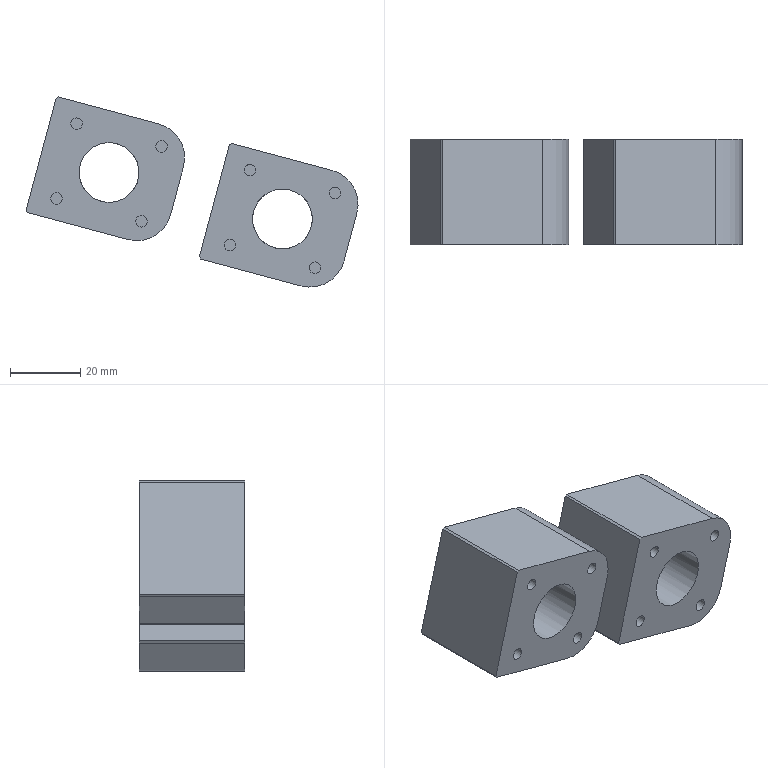Part | NX | 2 solids | 42 faces | box 94.322 x 30 x 54.017 mm | volume 58897 mm3 | plane 26 | cylinder 16 | commonest cylinder face diameters 3.3 x8 20 x4 17 x2 28.04 x2
STEP:
#1=CARTESIAN_POINT('',(618.06,-269.903,-13.791));
#2=VERTEX_POINT('',#1);
#3=CARTESIAN_POINT('',(604.04,-269.903,-13.791));
#4=DIRECTION('',(0.,-1.,0.));
#5=DIRECTION('',(1.,0.,0.000000051));
#6=AXIS2_PLACEMENT_3D('',#3,#4,#5);
#7=CIRCLE('',#6,14.02);
#8=EDGE_CURVE('',#2,#2,#7,.T.);
#9=ORIENTED_EDGE('',*,*,#8,.F.);
#10=EDGE_LOOP('',(#9));
#11=FACE_BOUND('',#10,.T.);
#12=CARTESIAN_POINT('',(612.54,-269.903,-13.791));
#13=VERTEX_POINT('',#12);
#14=CARTESIAN_POINT('',(604.04,-269.903,-13.791));
#15=DIRECTION('',(0.,-1.,0.));
#16=DIRECTION('',(1.,0.,0.));
#17=AXIS2_PLACEMENT_3D('',#14,#15,#16);
#18=CIRCLE('',#17,8.5);
#19=EDGE_CURVE('',#13,#13,#18,.T.);
#20=ORIENTED_EDGE('',*,*,#19,.T.);
#21=EDGE_LOOP('',(#20));
#22=FACE_BOUND('',#21,.T.);
#23=CARTESIAN_POINT('',(604.04,-269.903,-13.791));
#24=DIRECTION('',(0.,-1.,0.));
#25=DIRECTION('',(0.9659,0.,-0.2588));
#26=AXIS2_PLACEMENT_3D('',#23,#24,#25);
#27=PLANE('',#26);
#28=ADVANCED_FACE('',(#11,#22),#27,.F.);
#29=CARTESIAN_POINT('',(590.02,-262.903,-13.791));
#30=VERTEX_POINT('',#29);
#31=CARTESIAN_POINT('',(604.04,-262.903,-13.791));
#32=DIRECTION('',(0.,1.,0.));
#33=DIRECTION('',(-1.,0.,0.));
#34=AXIS2_PLACEMENT_3D('',#31,#32,#33);
#35=CIRCLE('',#34,14.02);
#36=EDGE_CURVE('',#30,#30,#35,.T.);
#37=ORIENTED_EDGE('',*,*,#36,.F.);
#38=EDGE_LOOP('',(#37));
#39=FACE_BOUND('',#38,.T.);
#40=CARTESIAN_POINT('',(589.604,-262.903,7.677));
#41=VERTEX_POINT('',#40);
#42=CARTESIAN_POINT('',(618.099,-262.903,0.04139));
#43=VERTEX_POINT('',#42);
#44=CARTESIAN_POINT('',(154.455,-262.903,124.275));
#45=DIRECTION('',(0.9659,0.,-0.2588));
#46=VECTOR('',#45,1000.);
#47=LINE('',#44,#46);
#48=EDGE_CURVE('',#41,#43,#47,.T.);
#49=ORIENTED_EDGE('',*,*,#48,.T.);
#50=CARTESIAN_POINT('',(625.17,-262.903,-12.206));
#51=VERTEX_POINT('',#50);
#52=CARTESIAN_POINT('',(615.511,-262.903,-9.618));
#53=DIRECTION('',(0.,1.,0.));
#54=DIRECTION('',(-1.,0.,0.));
#55=AXIS2_PLACEMENT_3D('',#52,#53,#54);
#56=CIRCLE('',#55,10.);
#57=EDGE_CURVE('',#43,#51,#56,.T.);
#58=ORIENTED_EDGE('',*,*,#57,.T.);
#59=CARTESIAN_POINT('',(621.547,-262.903,-25.729));
#60=VERTEX_POINT('',#59);
#61=CARTESIAN_POINT('',(622.064,-262.903,-23.797));
#62=DIRECTION('',(-0.2588,0.,-0.9659));
#63=VECTOR('',#62,1000.);
#64=LINE('',#61,#63);
#65=EDGE_CURVE('',#51,#60,#64,.T.);
#66=ORIENTED_EDGE('',*,*,#65,.T.);
#67=CARTESIAN_POINT('',(609.299,-262.903,-32.8));
#68=VERTEX_POINT('',#67);
#69=CARTESIAN_POINT('',(611.887,-262.903,-23.141));
#70=DIRECTION('',(0.,1.,0.));
#71=DIRECTION('',(-1.,0.,0.));
#72=AXIS2_PLACEMENT_3D('',#69,#70,#71);
#73=CIRCLE('',#72,10.);
#74=EDGE_CURVE('',#60,#68,#73,.T.);
#75=ORIENTED_EDGE('',*,*,#74,.T.);
#76=CARTESIAN_POINT('',(580.804,-262.903,-25.165));
#77=VERTEX_POINT('',#76);
#78=CARTESIAN_POINT('',(145.655,-262.903,91.433));
#79=DIRECTION('',(-0.9659,0.,0.2588));
#80=VECTOR('',#79,1000.);
#81=LINE('',#78,#80);
#82=EDGE_CURVE('',#68,#77,#81,.T.);
#83=ORIENTED_EDGE('',*,*,#82,.T.);
#84=CARTESIAN_POINT('',(580.451,-262.903,-24.553));
#85=VERTEX_POINT('',#84);
#86=CARTESIAN_POINT('',(417.286,-262.903,258.057));
#87=DIRECTION('',(-0.5,0.,0.866));
#88=VECTOR('',#87,1000.);
#89=LINE('',#86,#88);
#90=EDGE_CURVE('',#77,#85,#89,.T.);
#91=ORIENTED_EDGE('',*,*,#90,.T.);
#92=CARTESIAN_POINT('',(588.992,-262.903,7.323));
#93=VERTEX_POINT('',#92);
#94=CARTESIAN_POINT('',(583.427,-262.903,-13.444));
#95=DIRECTION('',(-0.2588,0.,-0.9659));
#96=VECTOR('',#95,1000.);
#97=LINE('',#94,#96);
#98=EDGE_CURVE('',#93,#85,#97,.T.);
#99=ORIENTED_EDGE('',*,*,#98,.F.);
#100=CARTESIAN_POINT('',(300.258,-262.903,-159.377));
#101=DIRECTION('',(0.866,0.,0.5));
#102=VECTOR('',#101,1000.);
#103=LINE('',#100,#102);
#104=EDGE_CURVE('',#93,#41,#103,.T.);
#105=ORIENTED_EDGE('',*,*,#104,.T.);
#106=EDGE_LOOP('',(#49,#58,#66,#75,#83,#91,#99,#105));
#107=FACE_BOUND('',#106,.T.);
#108=CARTESIAN_POINT('',(148.761,-262.903,103.024));
#109=DIRECTION('',(0.,1.,0.));
#110=DIRECTION('',(-0.9659,0.,0.2588));
#111=AXIS2_PLACEMENT_3D('',#108,#109,#110);
#112=PLANE('',#111);
#113=ADVANCED_FACE('',(#39,#107),#112,.T.);
#114=CARTESIAN_POINT('',(594.386,-292.903,-1.525));
#115=VERTEX_POINT('',#114);
#116=CARTESIAN_POINT('',(594.813,-292.903,0.06927));
#117=DIRECTION('',(0.,1.,0.));
#118=DIRECTION('',(-0.2588,0.,-0.9659));
#119=AXIS2_PLACEMENT_3D('',#116,#117,#118);
#120=CIRCLE('',#119,1.65);
#121=EDGE_CURVE('',#115,#115,#120,.T.);
#122=ORIENTED_EDGE('',*,*,#121,.T.);
#123=EDGE_LOOP('',(#122));
#124=FACE_BOUND('',#123,.T.);
#125=CARTESIAN_POINT('',(588.692,-292.903,-22.775));
#126=VERTEX_POINT('',#125);
#127=CARTESIAN_POINT('',(589.119,-292.903,-21.181));
#128=DIRECTION('',(0.,1.,0.));
#129=DIRECTION('',(-0.2588,0.,-0.9659));
#130=AXIS2_PLACEMENT_3D('',#127,#128,#129);
#131=CIRCLE('',#130,1.65);
#132=EDGE_CURVE('',#126,#126,#131,.T.);
#133=ORIENTED_EDGE('',*,*,#132,.T.);
#134=EDGE_LOOP('',(#133));
#135=FACE_BOUND('',#134,.T.);
#136=CARTESIAN_POINT('',(618.534,-292.903,-7.995));
#137=VERTEX_POINT('',#136);
#138=CARTESIAN_POINT('',(618.961,-292.903,-6.401));
#139=DIRECTION('',(0.,1.,0.));
#140=DIRECTION('',(-0.2588,0.,-0.9659));
#141=AXIS2_PLACEMENT_3D('',#138,#139,#140);
#142=CIRCLE('',#141,1.65);
#143=EDGE_CURVE('',#137,#137,#142,.T.);
#144=ORIENTED_EDGE('',*,*,#143,.T.);
#145=EDGE_LOOP('',(#144));
#146=FACE_BOUND('',#145,.T.);
#147=CARTESIAN_POINT('',(612.84,-292.903,-29.245));
#148=VERTEX_POINT('',#147);
#149=CARTESIAN_POINT('',(613.267,-292.903,-27.652));
#150=DIRECTION('',(0.,1.,0.));
#151=DIRECTION('',(-0.2588,0.,-0.9659));
#152=AXIS2_PLACEMENT_3D('',#149,#150,#151);
#153=CIRCLE('',#152,1.65);
#154=EDGE_CURVE('',#148,#148,#153,.T.);
#155=ORIENTED_EDGE('',*,*,#154,.T.);
#156=EDGE_LOOP('',(#155));
#157=FACE_BOUND('',#156,.T.);
#158=CARTESIAN_POINT('',(618.099,-292.903,0.04139));
#159=VERTEX_POINT('',#158);
#160=CARTESIAN_POINT('',(625.17,-292.903,-12.206));
#161=VERTEX_POINT('',#160);
#162=CARTESIAN_POINT('',(615.511,-292.903,-9.618));
#163=DIRECTION('',(0.,1.,0.));
#164=DIRECTION('',(0.,0.,1.));
#165=AXIS2_PLACEMENT_3D('',#162,#163,#164);
#166=CIRCLE('',#165,10.);
#167=EDGE_CURVE('',#159,#161,#166,.T.);
#168=ORIENTED_EDGE('',*,*,#167,.F.);
#169=CARTESIAN_POINT('',(589.604,-292.903,7.677));
#170=VERTEX_POINT('',#169);
#171=CARTESIAN_POINT('',(572.218,-292.903,12.335));
#172=DIRECTION('',(0.9659,0.,-0.2588));
#173=VECTOR('',#172,1000.);
#174=LINE('',#171,#173);
#175=EDGE_CURVE('',#170,#159,#174,.T.);
#176=ORIENTED_EDGE('',*,*,#175,.F.);
#177=CARTESIAN_POINT('',(588.992,-292.903,7.323));
#178=VERTEX_POINT('',#177);
#179=CARTESIAN_POINT('',(568.171,-292.903,-4.698));
#180=DIRECTION('',(0.866,0.,0.5));
#181=VECTOR('',#180,1000.);
#182=LINE('',#179,#181);
#183=EDGE_CURVE('',#178,#170,#182,.T.);
#184=ORIENTED_EDGE('',*,*,#183,.F.);
#185=CARTESIAN_POINT('',(580.451,-292.903,-24.553));
#186=VERTEX_POINT('',#185);
#187=CARTESIAN_POINT('',(584.721,-292.903,-8.615));
#188=DIRECTION('',(-0.2588,0.,-0.9659));
#189=VECTOR('',#188,1000.);
#190=LINE('',#187,#189);
#191=EDGE_CURVE('',#178,#186,#190,.T.);
#192=ORIENTED_EDGE('',*,*,#191,.T.);
#193=CARTESIAN_POINT('',(580.804,-292.903,-25.165));
#194=VERTEX_POINT('',#193);
#195=CARTESIAN_POINT('',(568.43,-292.903,-3.732));
#196=DIRECTION('',(-0.5,0.,0.866));
#197=VECTOR('',#196,1000.);
#198=LINE('',#195,#197);
#199=EDGE_CURVE('',#194,#186,#198,.T.);
#200=ORIENTED_EDGE('',*,*,#199,.F.);
#201=CARTESIAN_POINT('',(609.299,-292.903,-32.8));
#202=VERTEX_POINT('',#201);
#203=CARTESIAN_POINT('',(563.418,-292.903,-20.506));
#204=DIRECTION('',(-0.9659,0.,0.2588));
#205=VECTOR('',#204,1000.);
#206=LINE('',#203,#205);
#207=EDGE_CURVE('',#202,#194,#206,.T.);
#208=ORIENTED_EDGE('',*,*,#207,.F.);
#209=CARTESIAN_POINT('',(621.547,-292.903,-25.729));
#210=VERTEX_POINT('',#209);
#211=CARTESIAN_POINT('',(611.887,-292.903,-23.141));
#212=DIRECTION('',(0.,1.,0.));
#213=DIRECTION('',(0.,0.,1.));
#214=AXIS2_PLACEMENT_3D('',#211,#212,#213);
#215=CIRCLE('',#214,10.);
#216=EDGE_CURVE('',#210,#202,#215,.T.);
#217=ORIENTED_EDGE('',*,*,#216,.F.);
#218=CARTESIAN_POINT('',(623.358,-292.903,-18.968));
#219=DIRECTION('',(-0.2588,0.,-0.9659));
#220=VECTOR('',#219,1000.);
#221=LINE('',#218,#220);
#222=EDGE_CURVE('',#161,#210,#221,.T.);
#223=ORIENTED_EDGE('',*,*,#222,.F.);
#224=EDGE_LOOP('',(#168,#176,#184,#192,#200,#208,#217,#223));
#225=FACE_BOUND('',#224,.T.);
#226=CARTESIAN_POINT('',(604.04,-292.903,-5.291));
#227=VERTEX_POINT('',#226);
#228=CARTESIAN_POINT('',(604.04,-292.903,-13.791));
#229=DIRECTION('',(0.,1.,0.));
#230=DIRECTION('',(0.,0.,1.));
#231=AXIS2_PLACEMENT_3D('',#228,#229,#230);
#232=CIRCLE('',#231,8.5);
#233=EDGE_CURVE('',#227,#227,#232,.T.);
#234=ORIENTED_EDGE('',*,*,#233,.T.);
#235=EDGE_LOOP('',(#234));
#236=FACE_BOUND('',#235,.T.);
#237=CARTESIAN_POINT('',(567.818,-292.903,-4.085));
#238=DIRECTION('',(0.,1.,0.));
#239=DIRECTION('',(-0.2588,0.,-0.9659));
#240=AXIS2_PLACEMENT_3D('',#237,#238,#239);
#241=PLANE('',#240);
#242=ADVANCED_FACE('',(#124,#135,#146,#157,#225,#236),#241,.F.);
#243=ORIENTED_EDGE('',*,*,#57,.F.);
#244=CARTESIAN_POINT('',(618.099,-277.903,0.04139));
#245=DIRECTION('',(0.,-1.,0.));
#246=VECTOR('',#245,1000.);
#247=LINE('',#244,#246);
#248=EDGE_CURVE('',#43,#159,#247,.T.);
#249=ORIENTED_EDGE('',*,*,#248,.T.);
#250=ORIENTED_EDGE('',*,*,#167,.T.);
#251=CARTESIAN_POINT('',(625.17,-279.903,-12.206));
#252=DIRECTION('',(0.,1.,0.));
#253=VECTOR('',#252,1000.);
#254=LINE('',#251,#253);
#255=EDGE_CURVE('',#161,#51,#254,.T.);
#256=ORIENTED_EDGE('',*,*,#255,.T.);
#257=EDGE_LOOP('',(#243,#249,#250,#256));
#258=FACE_BOUND('',#257,.T.);
#259=CARTESIAN_POINT('',(615.511,-279.903,-9.618));
#260=DIRECTION('',(0.,1.,0.));
#261=DIRECTION('',(0.9659,0.,-0.2588));
#262=AXIS2_PLACEMENT_3D('',#259,#260,#261);
#263=CYLINDRICAL_SURFACE('',#262,10.);
#264=ADVANCED_FACE('',(#258),#263,.T.);
#265=ORIENTED_EDGE('',*,*,#65,.F.);
#266=ORIENTED_EDGE('',*,*,#255,.F.);
#267=ORIENTED_EDGE('',*,*,#222,.T.);
#268=CARTESIAN_POINT('',(621.547,-279.903,-25.729));
#269=DIRECTION('',(0.,-1.,0.));
#270=VECTOR('',#269,1000.);
#271=LINE('',#268,#270);
#272=EDGE_CURVE('',#60,#210,#271,.T.);
#273=ORIENTED_EDGE('',*,*,#272,.F.);
#274=EDGE_LOOP('',(#265,#266,#267,#273));
#275=FACE_BOUND('',#274,.T.);
#276=CARTESIAN_POINT('',(622.064,-279.903,-23.797));
#277=DIRECTION('',(0.9659,0.,-0.2588));
#278=DIRECTION('',(0.,1.,0.));
#279=AXIS2_PLACEMENT_3D('',#276,#277,#278);
#280=PLANE('',#279);
#281=ADVANCED_FACE('',(#275),#280,.T.);
#282=ORIENTED_EDGE('',*,*,#74,.F.);
#283=ORIENTED_EDGE('',*,*,#272,.T.);
#284=ORIENTED_EDGE('',*,*,#216,.T.);
#285=CARTESIAN_POINT('',(609.299,-277.903,-32.8));
#286=DIRECTION('',(0.,1.,0.));
#287=VECTOR('',#286,1000.);
#288=LINE('',#285,#287);
#289=EDGE_CURVE('',#202,#68,#288,.T.);
#290=ORIENTED_EDGE('',*,*,#289,.T.);
#291=EDGE_LOOP('',(#282,#283,#284,#290));
#292=FACE_BOUND('',#291,.T.);
#293=CARTESIAN_POINT('',(611.887,-279.903,-23.141));
#294=DIRECTION('',(0.,-1.,0.));
#295=DIRECTION('',(-0.9659,0.,0.2588));
#296=AXIS2_PLACEMENT_3D('',#293,#294,#295);
#297=CYLINDRICAL_SURFACE('',#296,10.);
#298=ADVANCED_FACE('',(#292),#297,.T.);
#299=ORIENTED_EDGE('',*,*,#82,.F.);
#300=ORIENTED_EDGE('',*,*,#289,.F.);
#301=ORIENTED_EDGE('',*,*,#207,.T.);
#302=CARTESIAN_POINT('',(580.804,-262.903,-25.165));
#303=DIRECTION('',(0.,1.,0.));
#304=VECTOR('',#303,1000.);
#305=LINE('',#302,#304);
#306=EDGE_CURVE('',#194,#77,#305,.T.);
#307=ORIENTED_EDGE('',*,*,#306,.T.);
#308=EDGE_LOOP('',(#299,#300,#301,#307));
#309=FACE_BOUND('',#308,.T.);
#310=CARTESIAN_POINT('',(383.273,-277.903,27.764));
#311=DIRECTION('',(-0.2588,0.,-0.9659));
#312=DIRECTION('',(0.,-1.,0.));
#313=AXIS2_PLACEMENT_3D('',#310,#311,#312);
#314=PLANE('',#313);
#315=ADVANCED_FACE('',(#309),#314,.T.);
#316=ORIENTED_EDGE('',*,*,#90,.F.);
#317=ORIENTED_EDGE('',*,*,#306,.F.);
#318=ORIENTED_EDGE('',*,*,#199,.T.);
#319=CARTESIAN_POINT('',(580.451,-292.903,-24.553));
#320=DIRECTION('',(0.,-1.,0.));
#321=VECTOR('',#320,1000.);
#322=LINE('',#319,#321);
#323=EDGE_CURVE('',#85,#186,#322,.T.);
#324=ORIENTED_EDGE('',*,*,#323,.F.);
#325=EDGE_LOOP('',(#316,#317,#318,#324));
#326=FACE_BOUND('',#325,.T.);
#327=CARTESIAN_POINT('',(580.451,-269.903,-24.553));
#328=DIRECTION('',(-0.866,0.,-0.5));
#329=DIRECTION('',(0.,1.,0.));
#330=AXIS2_PLACEMENT_3D('',#327,#328,#329);
#331=PLANE('',#330);
#332=ADVANCED_FACE('',(#326),#331,.T.);
#333=CARTESIAN_POINT('',(588.992,-262.903,7.323));
#334=DIRECTION('',(0.,1.,0.));
#335=VECTOR('',#334,1000.);
#336=LINE('',#333,#335);
#337=EDGE_CURVE('',#178,#93,#336,.T.);
#338=ORIENTED_EDGE('',*,*,#337,.T.);
#339=ORIENTED_EDGE('',*,*,#98,.T.);
#340=ORIENTED_EDGE('',*,*,#323,.T.);
#341=ORIENTED_EDGE('',*,*,#191,.F.);
#342=EDGE_LOOP('',(#338,#339,#340,#341));
#343=FACE_BOUND('',#342,.T.);
#344=CARTESIAN_POINT('',(584.721,-269.903,-8.615));
#345=DIRECTION('',(0.9659,0.,-0.2588));
#346=DIRECTION('',(0.2588,0.,0.9659));
#347=AXIS2_PLACEMENT_3D('',#344,#345,#346);
#348=PLANE('',#347);
#349=ADVANCED_FACE('',(#343),#348,.F.);
#350=ORIENTED_EDGE('',*,*,#104,.F.);
#351=ORIENTED_EDGE('',*,*,#337,.F.);
#352=ORIENTED_EDGE('',*,*,#183,.T.);
#353=CARTESIAN_POINT('',(589.604,-292.903,7.677));
#354=DIRECTION('',(0.,-1.,0.));
#355=VECTOR('',#354,1000.);
#356=LINE('',#353,#355);
#357=EDGE_CURVE('',#41,#170,#356,.T.);
#358=ORIENTED_EDGE('',*,*,#357,.F.);
#359=EDGE_LOOP('',(#350,#351,#352,#358));
#360=FACE_BOUND('',#359,.T.);
#361=CARTESIAN_POINT('',(589.604,-277.903,7.677));
#362=DIRECTION('',(-0.5,0.,0.866));
#363=DIRECTION('',(0.,1.,0.));
#364=AXIS2_PLACEMENT_3D('',#361,#362,#363);
#365=PLANE('',#364);
#366=ADVANCED_FACE('',(#360),#365,.T.);
#367=ORIENTED_EDGE('',*,*,#48,.F.);
#368=ORIENTED_EDGE('',*,*,#357,.T.);
#369=ORIENTED_EDGE('',*,*,#175,.T.);
#370=ORIENTED_EDGE('',*,*,#248,.F.);
#371=EDGE_LOOP('',(#367,#368,#369,#370));
#372=FACE_BOUND('',#371,.T.);
#373=CARTESIAN_POINT('',(392.072,-277.903,60.605));
#374=DIRECTION('',(0.2588,0.,0.9659));
#375=DIRECTION('',(0.,1.,0.));
#376=AXIS2_PLACEMENT_3D('',#373,#374,#375);
#377=PLANE('',#376);
#378=ADVANCED_FACE('',(#372),#377,.T.);
#379=ORIENTED_EDGE('',*,*,#121,.F.);
#380=EDGE_LOOP('',(#379));
#381=FACE_BOUND('',#380,.T.);
#382=CARTESIAN_POINT('',(594.813,-277.903,1.719));
#383=VERTEX_POINT('',#382);
#384=CARTESIAN_POINT('',(594.813,-277.903,0.06927));
#385=DIRECTION('',(0.,-1.,0.));
#386=DIRECTION('',(0.,0.,1.));
#387=AXIS2_PLACEMENT_3D('',#384,#385,#386);
#388=CIRCLE('',#387,1.65);
#389=EDGE_CURVE('',#383,#383,#388,.T.);
#390=ORIENTED_EDGE('',*,*,#389,.F.);
#391=EDGE_LOOP('',(#390));
#392=FACE_BOUND('',#391,.T.);
#393=CARTESIAN_POINT('',(594.813,-292.903,0.06927));
#394=DIRECTION('',(0.,1.,0.));
#395=DIRECTION('',(-0.2588,0.,-0.9659));
#396=AXIS2_PLACEMENT_3D('',#393,#394,#395);
#397=CYLINDRICAL_SURFACE('',#396,1.65);
#398=ADVANCED_FACE('',(#381,#392),#397,.F.);
#399=ORIENTED_EDGE('',*,*,#389,.T.);
#400=EDGE_LOOP('',(#399));
#401=FACE_BOUND('',#400,.T.);
#402=CARTESIAN_POINT('',(589.119,-277.903,-21.181));
#403=DIRECTION('',(0.,1.,0.));
#404=DIRECTION('',(-0.2588,0.,-0.9659));
#405=AXIS2_PLACEMENT_3D('',#402,#403,#404);
#406=PLANE('',#405);
#407=ADVANCED_FACE('',(#401),#406,.F.);
#408=ORIENTED_EDGE('',*,*,#132,.F.);
#409=EDGE_LOOP('',(#408));
#410=FACE_BOUND('',#409,.T.);
#411=CARTESIAN_POINT('',(588.692,-277.903,-22.775));
#412=VERTEX_POINT('',#411);
#413=CARTESIAN_POINT('',(589.119,-277.903,-21.181));
#414=DIRECTION('',(0.,-1.,0.));
#415=DIRECTION('',(-0.2588,0.,-0.9659));
#416=AXIS2_PLACEMENT_3D('',#413,#414,#415);
#417=CIRCLE('',#416,1.65);
#418=EDGE_CURVE('',#412,#412,#417,.T.);
#419=ORIENTED_EDGE('',*,*,#418,.F.);
#420=EDGE_LOOP('',(#419));
#421=FACE_BOUND('',#420,.T.);
#422=CARTESIAN_POINT('',(589.119,-292.903,-21.181));
#423=DIRECTION('',(0.,1.,0.));
#424=DIRECTION('',(-0.2588,0.,-0.9659));
#425=AXIS2_PLACEMENT_3D('',#422,#423,#424);
#426=CYLINDRICAL_SURFACE('',#425,1.65);
#427=ADVANCED_FACE('',(#410,#421),#426,.F.);
#428=ORIENTED_EDGE('',*,*,#418,.T.);
#429=EDGE_LOOP('',(#428));
#430=FACE_BOUND('',#429,.T.);
#431=CARTESIAN_POINT('',(589.119,-277.903,-21.181));
#432=DIRECTION('',(0.,1.,0.));
#433=DIRECTION('',(-0.2588,0.,-0.9659));
#434=AXIS2_PLACEMENT_3D('',#431,#432,#433);
#435=PLANE('',#434);
#436=ADVANCED_FACE('',(#430),#435,.F.);
#437=ORIENTED_EDGE('',*,*,#143,.F.);
#438=EDGE_LOOP('',(#437));
#439=FACE_BOUND('',#438,.T.);
#440=CARTESIAN_POINT('',(618.961,-277.903,-4.751));
#441=VERTEX_POINT('',#440);
#442=CARTESIAN_POINT('',(618.961,-277.903,-6.401));
#443=DIRECTION('',(0.,-1.,0.));
#444=DIRECTION('',(0.,0.,1.));
#445=AXIS2_PLACEMENT_3D('',#442,#443,#444);
#446=CIRCLE('',#445,1.65);
#447=EDGE_CURVE('',#441,#441,#446,.T.);
#448=ORIENTED_EDGE('',*,*,#447,.F.);
#449=EDGE_LOOP('',(#448));
#450=FACE_BOUND('',#449,.T.);
#451=CARTESIAN_POINT('',(618.961,-292.903,-6.401));
#452=DIRECTION('',(0.,1.,0.));
#453=DIRECTION('',(-0.2588,0.,-0.9659));
#454=AXIS2_PLACEMENT_3D('',#451,#452,#453);
#455=CYLINDRICAL_SURFACE('',#454,1.65);
#456=ADVANCED_FACE('',(#439,#450),#455,.F.);
#457=ORIENTED_EDGE('',*,*,#447,.T.);
#458=EDGE_LOOP('',(#457));
#459=FACE_BOUND('',#458,.T.);
#460=CARTESIAN_POINT('',(589.119,-277.903,-21.181));
#461=DIRECTION('',(0.,1.,0.));
#462=DIRECTION('',(-0.2588,0.,-0.9659));
#463=AXIS2_PLACEMENT_3D('',#460,#461,#462);
#464=PLANE('',#463);
#465=ADVANCED_FACE('',(#459),#464,.F.);
#466=ORIENTED_EDGE('',*,*,#154,.F.);
#467=EDGE_LOOP('',(#466));
#468=FACE_BOUND('',#467,.T.);
#469=CARTESIAN_POINT('',(613.267,-277.903,-26.002));
#470=VERTEX_POINT('',#469);
#471=CARTESIAN_POINT('',(613.267,-277.903,-27.652));
#472=DIRECTION('',(0.,-1.,0.));
#473=DIRECTION('',(0.,0.,1.));
#474=AXIS2_PLACEMENT_3D('',#471,#472,#473);
#475=CIRCLE('',#474,1.65);
#476=EDGE_CURVE('',#470,#470,#475,.T.);
#477=ORIENTED_EDGE('',*,*,#476,.F.);
#478=EDGE_LOOP('',(#477));
#479=FACE_BOUND('',#478,.T.);
#480=CARTESIAN_POINT('',(613.267,-292.903,-27.652));
#481=DIRECTION('',(0.,1.,0.));
#482=DIRECTION('',(-0.2588,0.,-0.9659));
#483=AXIS2_PLACEMENT_3D('',#480,#481,#482);
#484=CYLINDRICAL_SURFACE('',#483,1.65);
#485=ADVANCED_FACE('',(#468,#479),#484,.F.);
#486=ORIENTED_EDGE('',*,*,#476,.T.);
#487=EDGE_LOOP('',(#486));
#488=FACE_BOUND('',#487,.T.);
#489=CARTESIAN_POINT('',(589.119,-277.903,-21.181));
#490=DIRECTION('',(0.,1.,0.));
#491=DIRECTION('',(-0.2588,0.,-0.9659));
#492=AXIS2_PLACEMENT_3D('',#489,#490,#491);
#493=PLANE('',#492);
#494=ADVANCED_FACE('',(#488),#493,.F.);
#495=ORIENTED_EDGE('',*,*,#233,.F.);
#496=EDGE_LOOP('',(#495));
#497=FACE_BOUND('',#496,.T.);
#498=ORIENTED_EDGE('',*,*,#19,.F.);
#499=EDGE_LOOP('',(#498));
#500=FACE_BOUND('',#499,.T.);
#501=CARTESIAN_POINT('',(604.04,-284.903,-13.791));
#502=DIRECTION('',(0.,-1.,0.));
#503=DIRECTION('',(0.2588,0.,0.9659));
#504=AXIS2_PLACEMENT_3D('',#501,#502,#503);
#505=CYLINDRICAL_SURFACE('',#504,8.5);
#506=ADVANCED_FACE('',(#497,#500),#505,.F.);
#507=ORIENTED_EDGE('',*,*,#8,.T.);
#508=EDGE_LOOP('',(#507));
#509=FACE_BOUND('',#508,.T.);
#510=ORIENTED_EDGE('',*,*,#36,.T.);
#511=EDGE_LOOP('',(#510));
#512=FACE_BOUND('',#511,.T.);
#513=CARTESIAN_POINT('',(604.04,-269.903,-13.791));
#514=DIRECTION('',(0.,1.,0.));
#515=DIRECTION('',(-0.2588,0.,-0.9659));
#516=AXIS2_PLACEMENT_3D('',#513,#514,#515);
#517=CYLINDRICAL_SURFACE('',#516,14.02);
#518=ADVANCED_FACE('',(#509,#512),#517,.F.);
#519=CLOSED_SHELL('',(#28,#113,#242,#264,#281,#298,#315,#332,#349,#366,#378,#398,#407,#427,#436,#456,#465,#485,#494,#506,#518));
#520=MANIFOLD_SOLID_BREP('',#519);
#521=CARTESIAN_POINT('',(568.798,-269.903,-0.5914));
#522=VERTEX_POINT('',#521);
#523=CARTESIAN_POINT('',(554.778,-269.903,-0.5914));
#524=DIRECTION('',(0.,-1.,0.));
#525=DIRECTION('',(1.,0.,0.000000051));
#526=AXIS2_PLACEMENT_3D('',#523,#524,#525);
#527=CIRCLE('',#526,14.02);
#528=EDGE_CURVE('',#522,#522,#527,.T.);
#529=ORIENTED_EDGE('',*,*,#528,.F.);
#530=EDGE_LOOP('',(#529));
#531=FACE_BOUND('',#530,.T.);
#532=CARTESIAN_POINT('',(563.278,-269.903,-0.5914));
#533=VERTEX_POINT('',#532);
#534=CARTESIAN_POINT('',(554.778,-269.903,-0.5914));
#535=DIRECTION('',(0.,-1.,0.));
#536=DIRECTION('',(1.,0.,0.));
#537=AXIS2_PLACEMENT_3D('',#534,#535,#536);
#538=CIRCLE('',#537,8.5);
#539=EDGE_CURVE('',#533,#533,#538,.T.);
#540=ORIENTED_EDGE('',*,*,#539,.T.);
#541=EDGE_LOOP('',(#540));
#542=FACE_BOUND('',#541,.T.);
#543=CARTESIAN_POINT('',(554.778,-269.903,-0.5914));
#544=DIRECTION('',(0.,-1.,0.));
#545=DIRECTION('',(0.9659,0.,-0.2588));
#546=AXIS2_PLACEMENT_3D('',#543,#544,#545);
#547=PLANE('',#546);
#548=ADVANCED_FACE('',(#531,#542),#547,.F.);
#549=CARTESIAN_POINT('',(540.758,-262.903,-0.5914));
#550=VERTEX_POINT('',#549);
#551=CARTESIAN_POINT('',(554.778,-262.903,-0.5914));
#552=DIRECTION('',(0.,1.,0.));
#553=DIRECTION('',(-1.,0.,0.));
#554=AXIS2_PLACEMENT_3D('',#551,#552,#553);
#555=CIRCLE('',#554,14.02);
#556=EDGE_CURVE('',#550,#550,#555,.T.);
#557=ORIENTED_EDGE('',*,*,#556,.F.);
#558=EDGE_LOOP('',(#557));
#559=FACE_BOUND('',#558,.T.);
#560=CARTESIAN_POINT('',(540.342,-262.903,20.876));
#561=VERTEX_POINT('',#560);
#562=CARTESIAN_POINT('',(568.837,-262.903,13.241));
#563=VERTEX_POINT('',#562);
#564=CARTESIAN_POINT('',(105.193,-262.903,137.474));
#565=DIRECTION('',(0.9659,0.,-0.2588));
#566=VECTOR('',#565,1000.);
#567=LINE('',#564,#566);
#568=EDGE_CURVE('',#561,#563,#567,.T.);
#569=ORIENTED_EDGE('',*,*,#568,.T.);
#570=CARTESIAN_POINT('',(575.908,-262.903,0.9937));
#571=VERTEX_POINT('',#570);
#572=CARTESIAN_POINT('',(566.249,-262.903,3.582));
#573=DIRECTION('',(0.,1.,0.));
#574=DIRECTION('',(-1.,0.,0.));
#575=AXIS2_PLACEMENT_3D('',#572,#573,#574);
#576=CIRCLE('',#575,10.);
#577=EDGE_CURVE('',#563,#571,#576,.T.);
#578=ORIENTED_EDGE('',*,*,#577,.T.);
#579=CARTESIAN_POINT('',(572.285,-262.903,-12.529));
#580=VERTEX_POINT('',#579);
#581=CARTESIAN_POINT('',(572.802,-262.903,-10.597));
#582=DIRECTION('',(-0.2588,0.,-0.9659));
#583=VECTOR('',#582,1000.);
#584=LINE('',#581,#583);
#585=EDGE_CURVE('',#571,#580,#584,.T.);
#586=ORIENTED_EDGE('',*,*,#585,.T.);
#587=CARTESIAN_POINT('',(560.037,-262.903,-19.6));
#588=VERTEX_POINT('',#587);
#589=CARTESIAN_POINT('',(562.625,-262.903,-9.941));
#590=DIRECTION('',(0.,1.,0.));
#591=DIRECTION('',(-1.,0.,0.));
#592=AXIS2_PLACEMENT_3D('',#589,#590,#591);
#593=CIRCLE('',#592,10.);
#594=EDGE_CURVE('',#580,#588,#593,.T.);
#595=ORIENTED_EDGE('',*,*,#594,.T.);
#596=CARTESIAN_POINT('',(531.542,-262.903,-11.965));
#597=VERTEX_POINT('',#596);
#598=CARTESIAN_POINT('',(96.393,-262.903,104.633));
#599=DIRECTION('',(-0.9659,0.,0.2588));
#600=VECTOR('',#599,1000.);
#601=LINE('',#598,#600);
#602=EDGE_CURVE('',#588,#597,#601,.T.);
#603=ORIENTED_EDGE('',*,*,#602,.T.);
#604=CARTESIAN_POINT('',(531.189,-262.903,-11.353));
#605=VERTEX_POINT('',#604);
#606=CARTESIAN_POINT('',(368.024,-262.903,271.257));
#607=DIRECTION('',(-0.5,0.,0.866));
#608=VECTOR('',#607,1000.);
#609=LINE('',#606,#608);
#610=EDGE_CURVE('',#597,#605,#609,.T.);
#611=ORIENTED_EDGE('',*,*,#610,.T.);
#612=CARTESIAN_POINT('',(539.73,-262.903,20.523));
#613=VERTEX_POINT('',#612);
#614=CARTESIAN_POINT('',(534.165,-262.903,-0.2446));
#615=DIRECTION('',(-0.2588,0.,-0.9659));
#616=VECTOR('',#615,1000.);
#617=LINE('',#614,#616);
#618=EDGE_CURVE('',#613,#605,#617,.T.);
#619=ORIENTED_EDGE('',*,*,#618,.F.);
#620=CARTESIAN_POINT('',(250.996,-262.903,-146.178));
#621=DIRECTION('',(0.866,0.,0.5));
#622=VECTOR('',#621,1000.);
#623=LINE('',#620,#622);
#624=EDGE_CURVE('',#613,#561,#623,.T.);
#625=ORIENTED_EDGE('',*,*,#624,.T.);
#626=EDGE_LOOP('',(#569,#578,#586,#595,#603,#611,#619,#625));
#627=FACE_BOUND('',#626,.T.);
#628=CARTESIAN_POINT('',(99.499,-262.903,116.224));
#629=DIRECTION('',(0.,1.,0.));
#630=DIRECTION('',(-0.9659,0.,0.2588));
#631=AXIS2_PLACEMENT_3D('',#628,#629,#630);
#632=PLANE('',#631);
#633=ADVANCED_FACE('',(#559,#627),#632,.T.);
#634=CARTESIAN_POINT('',(545.124,-292.903,11.675));
#635=VERTEX_POINT('',#634);
#636=CARTESIAN_POINT('',(545.551,-292.903,13.269));
#637=DIRECTION('',(0.,1.,0.));
#638=DIRECTION('',(-0.2588,0.,-0.9659));
#639=AXIS2_PLACEMENT_3D('',#636,#637,#638);
#640=CIRCLE('',#639,1.65);
#641=EDGE_CURVE('',#635,#635,#640,.T.);
#642=ORIENTED_EDGE('',*,*,#641,.T.);
#643=EDGE_LOOP('',(#642));
#644=FACE_BOUND('',#643,.T.);
#645=CARTESIAN_POINT('',(539.43,-292.903,-9.575));
#646=VERTEX_POINT('',#645);
#647=CARTESIAN_POINT('',(539.857,-292.903,-7.981));
#648=DIRECTION('',(0.,1.,0.));
#649=DIRECTION('',(-0.2588,0.,-0.9659));
#650=AXIS2_PLACEMENT_3D('',#647,#648,#649);
#651=CIRCLE('',#650,1.65);
#652=EDGE_CURVE('',#646,#646,#651,.T.);
#653=ORIENTED_EDGE('',*,*,#652,.T.);
#654=EDGE_LOOP('',(#653));
#655=FACE_BOUND('',#654,.T.);
#656=CARTESIAN_POINT('',(569.272,-292.903,5.205));
#657=VERTEX_POINT('',#656);
#658=CARTESIAN_POINT('',(569.699,-292.903,6.799));
#659=DIRECTION('',(0.,1.,0.));
#660=DIRECTION('',(-0.2588,0.,-0.9659));
#661=AXIS2_PLACEMENT_3D('',#658,#659,#660);
#662=CIRCLE('',#661,1.65);
#663=EDGE_CURVE('',#657,#657,#662,.T.);
#664=ORIENTED_EDGE('',*,*,#663,.T.);
#665=EDGE_LOOP('',(#664));
#666=FACE_BOUND('',#665,.T.);
#667=CARTESIAN_POINT('',(563.578,-292.903,-16.046));
#668=VERTEX_POINT('',#667);
#669=CARTESIAN_POINT('',(564.005,-292.903,-14.452));
#670=DIRECTION('',(0.,1.,0.));
#671=DIRECTION('',(-0.2588,0.,-0.9659));
#672=AXIS2_PLACEMENT_3D('',#669,#670,#671);
#673=CIRCLE('',#672,1.65);
#674=EDGE_CURVE('',#668,#668,#673,.T.);
#675=ORIENTED_EDGE('',*,*,#674,.T.);
#676=EDGE_LOOP('',(#675));
#677=FACE_BOUND('',#676,.T.);
#678=CARTESIAN_POINT('',(568.837,-292.903,13.241));
#679=VERTEX_POINT('',#678);
#680=CARTESIAN_POINT('',(575.908,-292.903,0.9937));
#681=VERTEX_POINT('',#680);
#682=CARTESIAN_POINT('',(566.249,-292.903,3.582));
#683=DIRECTION('',(0.,1.,0.));
#684=DIRECTION('',(0.,0.,1.));
#685=AXIS2_PLACEMENT_3D('',#682,#683,#684);
#686=CIRCLE('',#685,10.);
#687=EDGE_CURVE('',#679,#681,#686,.T.);
#688=ORIENTED_EDGE('',*,*,#687,.F.);
#689=CARTESIAN_POINT('',(540.342,-292.903,20.876));
#690=VERTEX_POINT('',#689);
#691=CARTESIAN_POINT('',(522.955,-292.903,25.535));
#692=DIRECTION('',(0.9659,0.,-0.2588));
#693=VECTOR('',#692,1000.);
#694=LINE('',#691,#693);
#695=EDGE_CURVE('',#690,#679,#694,.T.);
#696=ORIENTED_EDGE('',*,*,#695,.F.);
#697=CARTESIAN_POINT('',(539.73,-292.903,20.523));
#698=VERTEX_POINT('',#697);
#699=CARTESIAN_POINT('',(518.909,-292.903,8.502));
#700=DIRECTION('',(0.866,0.,0.5));
#701=VECTOR('',#700,1000.);
#702=LINE('',#699,#701);
#703=EDGE_CURVE('',#698,#690,#702,.T.);
#704=ORIENTED_EDGE('',*,*,#703,.F.);
#705=CARTESIAN_POINT('',(531.189,-292.903,-11.353));
#706=VERTEX_POINT('',#705);
#707=CARTESIAN_POINT('',(535.459,-292.903,4.585));
#708=DIRECTION('',(-0.2588,0.,-0.9659));
#709=VECTOR('',#708,1000.);
#710=LINE('',#707,#709);
#711=EDGE_CURVE('',#698,#706,#710,.T.);
#712=ORIENTED_EDGE('',*,*,#711,.T.);
#713=CARTESIAN_POINT('',(531.542,-292.903,-11.965));
#714=VERTEX_POINT('',#713);
#715=CARTESIAN_POINT('',(519.168,-292.903,9.468));
#716=DIRECTION('',(-0.5,0.,0.866));
#717=VECTOR('',#716,1000.);
#718=LINE('',#715,#717);
#719=EDGE_CURVE('',#714,#706,#718,.T.);
#720=ORIENTED_EDGE('',*,*,#719,.F.);
#721=CARTESIAN_POINT('',(560.037,-292.903,-19.6));
#722=VERTEX_POINT('',#721);
#723=CARTESIAN_POINT('',(514.156,-292.903,-7.306));
#724=DIRECTION('',(-0.9659,0.,0.2588));
#725=VECTOR('',#724,1000.);
#726=LINE('',#723,#725);
#727=EDGE_CURVE('',#722,#714,#726,.T.);
#728=ORIENTED_EDGE('',*,*,#727,.F.);
#729=CARTESIAN_POINT('',(572.285,-292.903,-12.529));
#730=VERTEX_POINT('',#729);
#731=CARTESIAN_POINT('',(562.625,-292.903,-9.941));
#732=DIRECTION('',(0.,1.,0.));
#733=DIRECTION('',(0.,0.,1.));
#734=AXIS2_PLACEMENT_3D('',#731,#732,#733);
#735=CIRCLE('',#734,10.);
#736=EDGE_CURVE('',#730,#722,#735,.T.);
#737=ORIENTED_EDGE('',*,*,#736,.F.);
#738=CARTESIAN_POINT('',(574.096,-292.903,-5.768));
#739=DIRECTION('',(-0.2588,0.,-0.9659));
#740=VECTOR('',#739,1000.);
#741=LINE('',#738,#740);
#742=EDGE_CURVE('',#681,#730,#741,.T.);
#743=ORIENTED_EDGE('',*,*,#742,.F.);
#744=EDGE_LOOP('',(#688,#696,#704,#712,#720,#728,#737,#743));
#745=FACE_BOUND('',#744,.T.);
#746=CARTESIAN_POINT('',(554.778,-292.903,7.909));
#747=VERTEX_POINT('',#746);
#748=CARTESIAN_POINT('',(554.778,-292.903,-0.5914));
#749=DIRECTION('',(0.,1.,0.));
#750=DIRECTION('',(0.,0.,1.));
#751=AXIS2_PLACEMENT_3D('',#748,#749,#750);
#752=CIRCLE('',#751,8.5);
#753=EDGE_CURVE('',#747,#747,#752,.T.);
#754=ORIENTED_EDGE('',*,*,#753,.T.);
#755=EDGE_LOOP('',(#754));
#756=FACE_BOUND('',#755,.T.);
#757=CARTESIAN_POINT('',(518.556,-292.903,9.114));
#758=DIRECTION('',(0.,1.,0.));
#759=DIRECTION('',(-0.2588,0.,-0.9659));
#760=AXIS2_PLACEMENT_3D('',#757,#758,#759);
#761=PLANE('',#760);
#762=ADVANCED_FACE('',(#644,#655,#666,#677,#745,#756),#761,.F.);
#763=ORIENTED_EDGE('',*,*,#577,.F.);
#764=CARTESIAN_POINT('',(568.837,-277.903,13.241));
#765=DIRECTION('',(0.,-1.,0.));
#766=VECTOR('',#765,1000.);
#767=LINE('',#764,#766);
#768=EDGE_CURVE('',#563,#679,#767,.T.);
#769=ORIENTED_EDGE('',*,*,#768,.T.);
#770=ORIENTED_EDGE('',*,*,#687,.T.);
#771=CARTESIAN_POINT('',(575.908,-279.903,0.9937));
#772=DIRECTION('',(0.,1.,0.));
#773=VECTOR('',#772,1000.);
#774=LINE('',#771,#773);
#775=EDGE_CURVE('',#681,#571,#774,.T.);
#776=ORIENTED_EDGE('',*,*,#775,.T.);
#777=EDGE_LOOP('',(#763,#769,#770,#776));
#778=FACE_BOUND('',#777,.T.);
#779=CARTESIAN_POINT('',(566.249,-279.903,3.582));
#780=DIRECTION('',(0.,1.,0.));
#781=DIRECTION('',(0.9659,0.,-0.2588));
#782=AXIS2_PLACEMENT_3D('',#779,#780,#781);
#783=CYLINDRICAL_SURFACE('',#782,10.);
#784=ADVANCED_FACE('',(#778),#783,.T.);
#785=ORIENTED_EDGE('',*,*,#585,.F.);
#786=ORIENTED_EDGE('',*,*,#775,.F.);
#787=ORIENTED_EDGE('',*,*,#742,.T.);
#788=CARTESIAN_POINT('',(572.285,-279.903,-12.529));
#789=DIRECTION('',(0.,-1.,0.));
#790=VECTOR('',#789,1000.);
#791=LINE('',#788,#790);
#792=EDGE_CURVE('',#580,#730,#791,.T.);
#793=ORIENTED_EDGE('',*,*,#792,.F.);
#794=EDGE_LOOP('',(#785,#786,#787,#793));
#795=FACE_BOUND('',#794,.T.);
#796=CARTESIAN_POINT('',(572.802,-279.903,-10.597));
#797=DIRECTION('',(0.9659,0.,-0.2588));
#798=DIRECTION('',(0.,1.,0.));
#799=AXIS2_PLACEMENT_3D('',#796,#797,#798);
#800=PLANE('',#799);
#801=ADVANCED_FACE('',(#795),#800,.T.);
#802=ORIENTED_EDGE('',*,*,#594,.F.);
#803=ORIENTED_EDGE('',*,*,#792,.T.);
#804=ORIENTED_EDGE('',*,*,#736,.T.);
#805=CARTESIAN_POINT('',(560.037,-277.903,-19.6));
#806=DIRECTION('',(0.,1.,0.));
#807=VECTOR('',#806,1000.);
#808=LINE('',#805,#807);
#809=EDGE_CURVE('',#722,#588,#808,.T.);
#810=ORIENTED_EDGE('',*,*,#809,.T.);
#811=EDGE_LOOP('',(#802,#803,#804,#810));
#812=FACE_BOUND('',#811,.T.);
#813=CARTESIAN_POINT('',(562.625,-279.903,-9.941));
#814=DIRECTION('',(0.,-1.,0.));
#815=DIRECTION('',(-0.9659,0.,0.2588));
#816=AXIS2_PLACEMENT_3D('',#813,#814,#815);
#817=CYLINDRICAL_SURFACE('',#816,10.);
#818=ADVANCED_FACE('',(#812),#817,.T.);
#819=ORIENTED_EDGE('',*,*,#602,.F.);
#820=ORIENTED_EDGE('',*,*,#809,.F.);
#821=ORIENTED_EDGE('',*,*,#727,.T.);
#822=CARTESIAN_POINT('',(531.542,-262.903,-11.965));
#823=DIRECTION('',(0.,1.,0.));
#824=VECTOR('',#823,1000.);
#825=LINE('',#822,#824);
#826=EDGE_CURVE('',#714,#597,#825,.T.);
#827=ORIENTED_EDGE('',*,*,#826,.T.);
#828=EDGE_LOOP('',(#819,#820,#821,#827));
#829=FACE_BOUND('',#828,.T.);
#830=CARTESIAN_POINT('',(334.01,-277.903,40.963));
#831=DIRECTION('',(-0.2588,0.,-0.9659));
#832=DIRECTION('',(0.,-1.,0.));
#833=AXIS2_PLACEMENT_3D('',#830,#831,#832);
#834=PLANE('',#833);
#835=ADVANCED_FACE('',(#829),#834,.T.);
#836=ORIENTED_EDGE('',*,*,#610,.F.);
#837=ORIENTED_EDGE('',*,*,#826,.F.);
#838=ORIENTED_EDGE('',*,*,#719,.T.);
#839=CARTESIAN_POINT('',(531.189,-292.903,-11.353));
#840=DIRECTION('',(0.,-1.,0.));
#841=VECTOR('',#840,1000.);
#842=LINE('',#839,#841);
#843=EDGE_CURVE('',#605,#706,#842,.T.);
#844=ORIENTED_EDGE('',*,*,#843,.F.);
#845=EDGE_LOOP('',(#836,#837,#838,#844));
#846=FACE_BOUND('',#845,.T.);
#847=CARTESIAN_POINT('',(531.189,-269.903,-11.353));
#848=DIRECTION('',(-0.866,0.,-0.5));
#849=DIRECTION('',(0.,1.,0.));
#850=AXIS2_PLACEMENT_3D('',#847,#848,#849);
#851=PLANE('',#850);
#852=ADVANCED_FACE('',(#846),#851,.T.);
#853=CARTESIAN_POINT('',(539.73,-262.903,20.523));
#854=DIRECTION('',(0.,1.,0.));
#855=VECTOR('',#854,1000.);
#856=LINE('',#853,#855);
#857=EDGE_CURVE('',#698,#613,#856,.T.);
#858=ORIENTED_EDGE('',*,*,#857,.T.);
#859=ORIENTED_EDGE('',*,*,#618,.T.);
#860=ORIENTED_EDGE('',*,*,#843,.T.);
#861=ORIENTED_EDGE('',*,*,#711,.F.);
#862=EDGE_LOOP('',(#858,#859,#860,#861));
#863=FACE_BOUND('',#862,.T.);
#864=CARTESIAN_POINT('',(535.459,-269.903,4.585));
#865=DIRECTION('',(0.9659,0.,-0.2588));
#866=DIRECTION('',(0.2588,0.,0.9659));
#867=AXIS2_PLACEMENT_3D('',#864,#865,#866);
#868=PLANE('',#867);
#869=ADVANCED_FACE('',(#863),#868,.F.);
#870=ORIENTED_EDGE('',*,*,#624,.F.);
#871=ORIENTED_EDGE('',*,*,#857,.F.);
#872=ORIENTED_EDGE('',*,*,#703,.T.);
#873=CARTESIAN_POINT('',(540.342,-292.903,20.876));
#874=DIRECTION('',(0.,-1.,0.));
#875=VECTOR('',#874,1000.);
#876=LINE('',#873,#875);
#877=EDGE_CURVE('',#561,#690,#876,.T.);
#878=ORIENTED_EDGE('',*,*,#877,.F.);
#879=EDGE_LOOP('',(#870,#871,#872,#878));
#880=FACE_BOUND('',#879,.T.);
#881=CARTESIAN_POINT('',(540.342,-277.903,20.876));
#882=DIRECTION('',(-0.5,0.,0.866));
#883=DIRECTION('',(0.,1.,0.));
#884=AXIS2_PLACEMENT_3D('',#881,#882,#883);
#885=PLANE('',#884);
#886=ADVANCED_FACE('',(#880),#885,.T.);
#887=ORIENTED_EDGE('',*,*,#568,.F.);
#888=ORIENTED_EDGE('',*,*,#877,.T.);
#889=ORIENTED_EDGE('',*,*,#695,.T.);
#890=ORIENTED_EDGE('',*,*,#768,.F.);
#891=EDGE_LOOP('',(#887,#888,#889,#890));
#892=FACE_BOUND('',#891,.T.);
#893=CARTESIAN_POINT('',(342.81,-277.903,73.805));
#894=DIRECTION('',(0.2588,0.,0.9659));
#895=DIRECTION('',(0.,1.,0.));
#896=AXIS2_PLACEMENT_3D('',#893,#894,#895);
#897=PLANE('',#896);
#898=ADVANCED_FACE('',(#892),#897,.T.);
#899=ORIENTED_EDGE('',*,*,#641,.F.);
#900=EDGE_LOOP('',(#899));
#901=FACE_BOUND('',#900,.T.);
#902=CARTESIAN_POINT('',(545.551,-277.903,14.919));
#903=VERTEX_POINT('',#902);
#904=CARTESIAN_POINT('',(545.551,-277.903,13.269));
#905=DIRECTION('',(0.,-1.,0.));
#906=DIRECTION('',(0.,0.,1.));
#907=AXIS2_PLACEMENT_3D('',#904,#905,#906);
#908=CIRCLE('',#907,1.65);
#909=EDGE_CURVE('',#903,#903,#908,.T.);
#910=ORIENTED_EDGE('',*,*,#909,.F.);
#911=EDGE_LOOP('',(#910));
#912=FACE_BOUND('',#911,.T.);
#913=CARTESIAN_POINT('',(545.551,-292.903,13.269));
#914=DIRECTION('',(0.,1.,0.));
#915=DIRECTION('',(-0.2588,0.,-0.9659));
#916=AXIS2_PLACEMENT_3D('',#913,#914,#915);
#917=CYLINDRICAL_SURFACE('',#916,1.65);
#918=ADVANCED_FACE('',(#901,#912),#917,.F.);
#919=ORIENTED_EDGE('',*,*,#909,.T.);
#920=EDGE_LOOP('',(#919));
#921=FACE_BOUND('',#920,.T.);
#922=CARTESIAN_POINT('',(539.857,-277.903,-7.981));
#923=DIRECTION('',(0.,1.,0.));
#924=DIRECTION('',(-0.2588,0.,-0.9659));
#925=AXIS2_PLACEMENT_3D('',#922,#923,#924);
#926=PLANE('',#925);
#927=ADVANCED_FACE('',(#921),#926,.F.);
#928=ORIENTED_EDGE('',*,*,#652,.F.);
#929=EDGE_LOOP('',(#928));
#930=FACE_BOUND('',#929,.T.);
#931=CARTESIAN_POINT('',(539.43,-277.903,-9.575));
#932=VERTEX_POINT('',#931);
#933=CARTESIAN_POINT('',(539.857,-277.903,-7.981));
#934=DIRECTION('',(0.,-1.,0.));
#935=DIRECTION('',(-0.2588,0.,-0.9659));
#936=AXIS2_PLACEMENT_3D('',#933,#934,#935);
#937=CIRCLE('',#936,1.65);
#938=EDGE_CURVE('',#932,#932,#937,.T.);
#939=ORIENTED_EDGE('',*,*,#938,.F.);
#940=EDGE_LOOP('',(#939));
#941=FACE_BOUND('',#940,.T.);
#942=CARTESIAN_POINT('',(539.857,-292.903,-7.981));
#943=DIRECTION('',(0.,1.,0.));
#944=DIRECTION('',(-0.2588,0.,-0.9659));
#945=AXIS2_PLACEMENT_3D('',#942,#943,#944);
#946=CYLINDRICAL_SURFACE('',#945,1.65);
#947=ADVANCED_FACE('',(#930,#941),#946,.F.);
#948=ORIENTED_EDGE('',*,*,#938,.T.);
#949=EDGE_LOOP('',(#948));
#950=FACE_BOUND('',#949,.T.);
#951=CARTESIAN_POINT('',(539.857,-277.903,-7.981));
#952=DIRECTION('',(0.,1.,0.));
#953=DIRECTION('',(-0.2588,0.,-0.9659));
#954=AXIS2_PLACEMENT_3D('',#951,#952,#953);
#955=PLANE('',#954);
#956=ADVANCED_FACE('',(#950),#955,.F.);
#957=ORIENTED_EDGE('',*,*,#663,.F.);
#958=EDGE_LOOP('',(#957));
#959=FACE_BOUND('',#958,.T.);
#960=CARTESIAN_POINT('',(569.699,-277.903,8.449));
#961=VERTEX_POINT('',#960);
#962=CARTESIAN_POINT('',(569.699,-277.903,6.799));
#963=DIRECTION('',(0.,-1.,0.));
#964=DIRECTION('',(0.,0.,1.));
#965=AXIS2_PLACEMENT_3D('',#962,#963,#964);
#966=CIRCLE('',#965,1.65);
#967=EDGE_CURVE('',#961,#961,#966,.T.);
#968=ORIENTED_EDGE('',*,*,#967,.F.);
#969=EDGE_LOOP('',(#968));
#970=FACE_BOUND('',#969,.T.);
#971=CARTESIAN_POINT('',(569.699,-292.903,6.799));
#972=DIRECTION('',(0.,1.,0.));
#973=DIRECTION('',(-0.2588,0.,-0.9659));
#974=AXIS2_PLACEMENT_3D('',#971,#972,#973);
#975=CYLINDRICAL_SURFACE('',#974,1.65);
#976=ADVANCED_FACE('',(#959,#970),#975,.F.);
#977=ORIENTED_EDGE('',*,*,#967,.T.);
#978=EDGE_LOOP('',(#977));
#979=FACE_BOUND('',#978,.T.);
#980=CARTESIAN_POINT('',(539.857,-277.903,-7.981));
#981=DIRECTION('',(0.,1.,0.));
#982=DIRECTION('',(-0.2588,0.,-0.9659));
#983=AXIS2_PLACEMENT_3D('',#980,#981,#982);
#984=PLANE('',#983);
#985=ADVANCED_FACE('',(#979),#984,.F.);
#986=ORIENTED_EDGE('',*,*,#674,.F.);
#987=EDGE_LOOP('',(#986));
#988=FACE_BOUND('',#987,.T.);
#989=CARTESIAN_POINT('',(564.005,-277.903,-12.802));
#990=VERTEX_POINT('',#989);
#991=CARTESIAN_POINT('',(564.005,-277.903,-14.452));
#992=DIRECTION('',(0.,-1.,0.));
#993=DIRECTION('',(0.,0.,1.));
#994=AXIS2_PLACEMENT_3D('',#991,#992,#993);
#995=CIRCLE('',#994,1.65);
#996=EDGE_CURVE('',#990,#990,#995,.T.);
#997=ORIENTED_EDGE('',*,*,#996,.F.);
#998=EDGE_LOOP('',(#997));
#999=FACE_BOUND('',#998,.T.);
#1000=CARTESIAN_POINT('',(564.005,-292.903,-14.452));
#1001=DIRECTION('',(0.,1.,0.));
#1002=DIRECTION('',(-0.2588,0.,-0.9659));
#1003=AXIS2_PLACEMENT_3D('',#1000,#1001,#1002);
#1004=CYLINDRICAL_SURFACE('',#1003,1.65);
#1005=ADVANCED_FACE('',(#988,#999),#1004,.F.);
#1006=ORIENTED_EDGE('',*,*,#996,.T.);
#1007=EDGE_LOOP('',(#1006));
#1008=FACE_BOUND('',#1007,.T.);
#1009=CARTESIAN_POINT('',(539.857,-277.903,-7.981));
#1010=DIRECTION('',(0.,1.,0.));
#1011=DIRECTION('',(-0.2588,0.,-0.9659));
#1012=AXIS2_PLACEMENT_3D('',#1009,#1010,#1011);
#1013=PLANE('',#1012);
#1014=ADVANCED_FACE('',(#1008),#1013,.F.);
#1015=ORIENTED_EDGE('',*,*,#753,.F.);
#1016=EDGE_LOOP('',(#1015));
#1017=FACE_BOUND('',#1016,.T.);
#1018=ORIENTED_EDGE('',*,*,#539,.F.);
#1019=EDGE_LOOP('',(#1018));
#1020=FACE_BOUND('',#1019,.T.);
#1021=CARTESIAN_POINT('',(554.778,-284.903,-0.5914));
#1022=DIRECTION('',(0.,-1.,0.));
#1023=DIRECTION('',(0.2588,0.,0.9659));
#1024=AXIS2_PLACEMENT_3D('',#1021,#1022,#1023);
#1025=CYLINDRICAL_SURFACE('',#1024,8.5);
#1026=ADVANCED_FACE('',(#1017,#1020),#1025,.F.);
#1027=ORIENTED_EDGE('',*,*,#528,.T.);
#1028=EDGE_LOOP('',(#1027));
#1029=FACE_BOUND('',#1028,.T.);
#1030=ORIENTED_EDGE('',*,*,#556,.T.);
#1031=EDGE_LOOP('',(#1030));
#1032=FACE_BOUND('',#1031,.T.);
#1033=CARTESIAN_POINT('',(554.778,-269.903,-0.5914));
#1034=DIRECTION('',(0.,1.,0.));
#1035=DIRECTION('',(-0.2588,0.,-0.9659));
#1036=AXIS2_PLACEMENT_3D('',#1033,#1034,#1035);
#1037=CYLINDRICAL_SURFACE('',#1036,14.02);
#1038=ADVANCED_FACE('',(#1029,#1032),#1037,.F.);
#1039=CLOSED_SHELL('',(#548,#633,#762,#784,#801,#818,#835,#852,#869,#886,#898,#918,#927,#947,#956,#976,#985,#1005,#1014,#1026,#1038));
#1040=MANIFOLD_SOLID_BREP('',#1039);
#1041=(LENGTH_UNIT()NAMED_UNIT(*)SI_UNIT(.MILLI.,.METRE.));
#1042=UNCERTAINTY_MEASURE_WITH_UNIT(LENGTH_MEASURE(0.00001),#1041,'','');
#1043=(NAMED_UNIT(*)PLANE_ANGLE_UNIT()SI_UNIT($,.RADIAN.));
#1044=(NAMED_UNIT(*)SI_UNIT($,.STERADIAN.)SOLID_ANGLE_UNIT());
#1045=(GEOMETRIC_REPRESENTATION_CONTEXT(3)GLOBAL_UNCERTAINTY_ASSIGNED_CONTEXT((#1042))GLOBAL_UNIT_ASSIGNED_CONTEXT((#1041,#1043,#1044))REPRESENTATION_CONTEXT('',''));
#1046=ADVANCED_BREP_SHAPE_REPRESENTATION('',(#520,#1040),#1045);